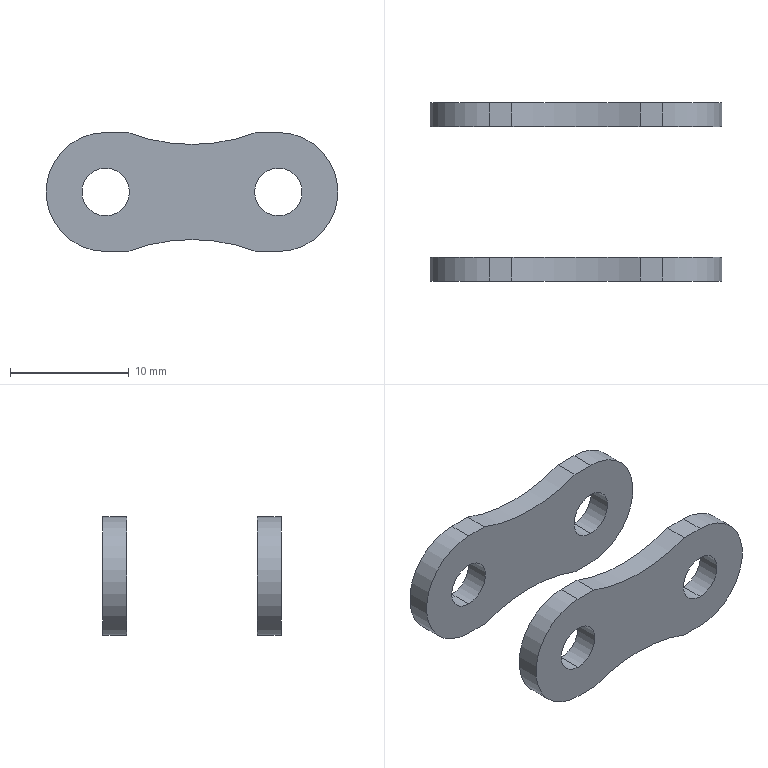Part | SolidWorks | features ICE 2, Extrusion 1 | 2 solids | 30 faces | box 24.52 x 15 x 10 mm | volume 736.592 mm3 | cylinder 18 | plane 12 | commonest cylinder face diameters 4 x8 30 x6 10 x4
STEP:
#1=CARTESIAN_POINT('',(7.26,13.,-4.));
#2=VERTEX_POINT('',#1);
#3=CARTESIAN_POINT('',(12.645,13.,-5.));
#4=VERTEX_POINT('',#3);
#5=CARTESIAN_POINT('',(7.26,13.,-19.));
#6=DIRECTION('',(0.,1.,0.));
#7=DIRECTION('',(0.,0.,1.));
#8=AXIS2_PLACEMENT_3D('',#5,#6,#7);
#9=CIRCLE('',#8,15.);
#10=EDGE_CURVE('',#2,#4,#9,.T.);
#11=ORIENTED_EDGE('',*,*,#10,.F.);
#12=CARTESIAN_POINT('',(7.26,15.,-4.));
#13=VERTEX_POINT('',#12);
#14=CARTESIAN_POINT('',(7.26,0.,-4.));
#15=DIRECTION('',(0.,1.,0.));
#16=VECTOR('',#15,1000.);
#17=LINE('',#14,#16);
#18=EDGE_CURVE('',#2,#13,#17,.T.);
#19=ORIENTED_EDGE('',*,*,#18,.T.);
#20=CARTESIAN_POINT('',(12.645,15.,-5.));
#21=VERTEX_POINT('',#20);
#22=CARTESIAN_POINT('',(7.26,15.,-19.));
#23=DIRECTION('',(0.,1.,0.));
#24=DIRECTION('',(0.,0.,1.));
#25=AXIS2_PLACEMENT_3D('',#22,#23,#24);
#26=CIRCLE('',#25,15.);
#27=EDGE_CURVE('',#13,#21,#26,.T.);
#28=ORIENTED_EDGE('',*,*,#27,.T.);
#29=CARTESIAN_POINT('',(12.645,0.,-5.));
#30=DIRECTION('',(0.,1.,0.));
#31=VECTOR('',#30,1000.);
#32=LINE('',#29,#31);
#33=EDGE_CURVE('',#4,#21,#32,.T.);
#34=ORIENTED_EDGE('',*,*,#33,.F.);
#35=EDGE_LOOP('',(#11,#19,#28,#34));
#36=FACE_OUTER_BOUND('',#35,.T.);
#37=CARTESIAN_POINT('',(7.26,0.,-19.));
#38=DIRECTION('',(0.,1.,0.));
#39=DIRECTION('',(0.,0.,1.));
#40=AXIS2_PLACEMENT_3D('',#37,#38,#39);
#41=CYLINDRICAL_SURFACE('',#40,15.);
#42=ADVANCED_FACE('',(#36),#41,.F.);
#43=CARTESIAN_POINT('',(14.52,15.,-2.));
#44=VERTEX_POINT('',#43);
#45=CARTESIAN_POINT('',(14.52,15.,2.));
#46=VERTEX_POINT('',#45);
#47=CARTESIAN_POINT('',(14.52,15.,0.));
#48=DIRECTION('',(0.,1.,0.));
#49=DIRECTION('',(0.,0.,1.));
#50=AXIS2_PLACEMENT_3D('',#47,#48,#49);
#51=CIRCLE('',#50,2.);
#52=EDGE_CURVE('',#44,#46,#51,.T.);
#53=ORIENTED_EDGE('',*,*,#52,.T.);
#54=CARTESIAN_POINT('',(14.52,13.,2.));
#55=VERTEX_POINT('',#54);
#56=CARTESIAN_POINT('',(14.52,15.,2.));
#57=DIRECTION('',(0.,-1.,0.));
#58=VECTOR('',#57,1000.);
#59=LINE('',#56,#58);
#60=EDGE_CURVE('',#46,#55,#59,.T.);
#61=ORIENTED_EDGE('',*,*,#60,.T.);
#62=CARTESIAN_POINT('',(14.52,13.,-2.));
#63=VERTEX_POINT('',#62);
#64=CARTESIAN_POINT('',(14.52,13.,0.));
#65=DIRECTION('',(0.,1.,0.));
#66=DIRECTION('',(0.,0.,1.));
#67=AXIS2_PLACEMENT_3D('',#64,#65,#66);
#68=CIRCLE('',#67,2.);
#69=EDGE_CURVE('',#63,#55,#68,.T.);
#70=ORIENTED_EDGE('',*,*,#69,.F.);
#71=CARTESIAN_POINT('',(14.52,15.,-2.));
#72=DIRECTION('',(0.,-1.,0.));
#73=VECTOR('',#72,1000.);
#74=LINE('',#71,#73);
#75=EDGE_CURVE('',#44,#63,#74,.T.);
#76=ORIENTED_EDGE('',*,*,#75,.F.);
#77=EDGE_LOOP('',(#53,#61,#70,#76));
#78=FACE_OUTER_BOUND('',#77,.T.);
#79=CARTESIAN_POINT('',(14.52,15.,0.));
#80=DIRECTION('',(0.,-1.,0.));
#81=DIRECTION('',(0.,0.,-1.));
#82=AXIS2_PLACEMENT_3D('',#79,#80,#81);
#83=CYLINDRICAL_SURFACE('',#82,2.);
#84=ADVANCED_FACE('',(#78),#83,.F.);
#85=CARTESIAN_POINT('',(0.,15.,-2.));
#86=VERTEX_POINT('',#85);
#87=CARTESIAN_POINT('',(0.,15.,2.));
#88=VERTEX_POINT('',#87);
#89=CARTESIAN_POINT('',(0.,15.,0.));
#90=DIRECTION('',(0.,1.,0.));
#91=DIRECTION('',(0.,0.,1.));
#92=AXIS2_PLACEMENT_3D('',#89,#90,#91);
#93=CIRCLE('',#92,2.);
#94=EDGE_CURVE('',#86,#88,#93,.T.);
#95=ORIENTED_EDGE('',*,*,#94,.T.);
#96=CARTESIAN_POINT('',(0.,13.,2.));
#97=VERTEX_POINT('',#96);
#98=CARTESIAN_POINT('',(0.,15.,2.));
#99=DIRECTION('',(0.,-1.,0.));
#100=VECTOR('',#99,1000.);
#101=LINE('',#98,#100);
#102=EDGE_CURVE('',#88,#97,#101,.T.);
#103=ORIENTED_EDGE('',*,*,#102,.T.);
#104=CARTESIAN_POINT('',(0.,13.,-2.));
#105=VERTEX_POINT('',#104);
#106=CARTESIAN_POINT('',(0.,13.,0.));
#107=DIRECTION('',(0.,1.,0.));
#108=DIRECTION('',(0.,0.,1.));
#109=AXIS2_PLACEMENT_3D('',#106,#107,#108);
#110=CIRCLE('',#109,2.);
#111=EDGE_CURVE('',#105,#97,#110,.T.);
#112=ORIENTED_EDGE('',*,*,#111,.F.);
#113=CARTESIAN_POINT('',(0.,15.,-2.));
#114=DIRECTION('',(0.,-1.,0.));
#115=VECTOR('',#114,1000.);
#116=LINE('',#113,#115);
#117=EDGE_CURVE('',#86,#105,#116,.T.);
#118=ORIENTED_EDGE('',*,*,#117,.F.);
#119=EDGE_LOOP('',(#95,#103,#112,#118));
#120=FACE_OUTER_BOUND('',#119,.T.);
#121=CARTESIAN_POINT('',(0.,15.,0.));
#122=DIRECTION('',(0.,-1.,0.));
#123=DIRECTION('',(0.,0.,-1.));
#124=AXIS2_PLACEMENT_3D('',#121,#122,#123);
#125=CYLINDRICAL_SURFACE('',#124,2.);
#126=ADVANCED_FACE('',(#120),#125,.F.);
#127=CARTESIAN_POINT('',(0.,13.,5.));
#128=VERTEX_POINT('',#127);
#129=CARTESIAN_POINT('',(1.875,13.,5.));
#130=VERTEX_POINT('',#129);
#131=CARTESIAN_POINT('',(0.,13.,5.));
#132=DIRECTION('',(1.,0.,0.));
#133=VECTOR('',#132,1000.);
#134=LINE('',#131,#133);
#135=EDGE_CURVE('',#128,#130,#134,.T.);
#136=ORIENTED_EDGE('',*,*,#135,.T.);
#137=CARTESIAN_POINT('',(1.875,15.,5.));
#138=VERTEX_POINT('',#137);
#139=CARTESIAN_POINT('',(1.875,0.,5.));
#140=DIRECTION('',(0.,1.,0.));
#141=VECTOR('',#140,1000.);
#142=LINE('',#139,#141);
#143=EDGE_CURVE('',#130,#138,#142,.T.);
#144=ORIENTED_EDGE('',*,*,#143,.T.);
#145=CARTESIAN_POINT('',(0.,15.,5.));
#146=VERTEX_POINT('',#145);
#147=CARTESIAN_POINT('',(0.,15.,5.));
#148=DIRECTION('',(1.,0.,0.));
#149=VECTOR('',#148,1000.);
#150=LINE('',#147,#149);
#151=EDGE_CURVE('',#146,#138,#150,.T.);
#152=ORIENTED_EDGE('',*,*,#151,.F.);
#153=CARTESIAN_POINT('',(0.,15.,5.));
#154=DIRECTION('',(0.,-1.,0.));
#155=VECTOR('',#154,1000.);
#156=LINE('',#153,#155);
#157=EDGE_CURVE('',#146,#128,#156,.T.);
#158=ORIENTED_EDGE('',*,*,#157,.T.);
#159=EDGE_LOOP('',(#136,#144,#152,#158));
#160=FACE_OUTER_BOUND('',#159,.T.);
#161=CARTESIAN_POINT('',(0.,15.,5.));
#162=DIRECTION('',(0.,0.,-1.));
#163=DIRECTION('',(-1.,0.,0.));
#164=AXIS2_PLACEMENT_3D('',#161,#162,#163);
#165=PLANE('',#164);
#166=ADVANCED_FACE('',(#160),#165,.F.);
#167=CARTESIAN_POINT('',(14.52,13.,-5.));
#168=VERTEX_POINT('',#167);
#169=CARTESIAN_POINT('',(0.,13.,-5.));
#170=DIRECTION('',(-1.,0.,0.));
#171=VECTOR('',#170,1000.);
#172=LINE('',#169,#171);
#173=EDGE_CURVE('',#168,#4,#172,.T.);
#174=ORIENTED_EDGE('',*,*,#173,.T.);
#175=ORIENTED_EDGE('',*,*,#33,.T.);
#176=CARTESIAN_POINT('',(14.52,15.,-5.));
#177=VERTEX_POINT('',#176);
#178=CARTESIAN_POINT('',(0.,15.,-5.));
#179=DIRECTION('',(-1.,0.,0.));
#180=VECTOR('',#179,1000.);
#181=LINE('',#178,#180);
#182=EDGE_CURVE('',#177,#21,#181,.T.);
#183=ORIENTED_EDGE('',*,*,#182,.F.);
#184=CARTESIAN_POINT('',(14.52,15.,-5.));
#185=DIRECTION('',(0.,-1.,0.));
#186=VECTOR('',#185,1000.);
#187=LINE('',#184,#186);
#188=EDGE_CURVE('',#177,#168,#187,.T.);
#189=ORIENTED_EDGE('',*,*,#188,.T.);
#190=EDGE_LOOP('',(#174,#175,#183,#189));
#191=FACE_OUTER_BOUND('',#190,.T.);
#192=CARTESIAN_POINT('',(0.,15.,-5.));
#193=DIRECTION('',(0.,0.,1.));
#194=DIRECTION('',(1.,0.,0.));
#195=AXIS2_PLACEMENT_3D('',#192,#193,#194);
#196=PLANE('',#195);
#197=ADVANCED_FACE('',(#191),#196,.F.);
#198=CARTESIAN_POINT('',(1.875,15.,-5.));
#199=VERTEX_POINT('',#198);
#200=CARTESIAN_POINT('',(7.26,15.,-19.));
#201=DIRECTION('',(0.,1.,0.));
#202=DIRECTION('',(0.,0.,1.));
#203=AXIS2_PLACEMENT_3D('',#200,#201,#202);
#204=CIRCLE('',#203,15.);
#205=EDGE_CURVE('',#199,#13,#204,.T.);
#206=ORIENTED_EDGE('',*,*,#205,.F.);
#207=CARTESIAN_POINT('',(0.,15.,-5.));
#208=VERTEX_POINT('',#207);
#209=CARTESIAN_POINT('',(0.,15.,-5.));
#210=DIRECTION('',(-1.,0.,0.));
#211=VECTOR('',#210,1000.);
#212=LINE('',#209,#211);
#213=EDGE_CURVE('',#199,#208,#212,.T.);
#214=ORIENTED_EDGE('',*,*,#213,.T.);
#215=CARTESIAN_POINT('',(0.,15.,0.));
#216=DIRECTION('',(0.,1.,0.));
#217=DIRECTION('',(0.,0.,1.));
#218=AXIS2_PLACEMENT_3D('',#215,#216,#217);
#219=CIRCLE('',#218,5.);
#220=EDGE_CURVE('',#208,#146,#219,.T.);
#221=ORIENTED_EDGE('',*,*,#220,.T.);
#222=ORIENTED_EDGE('',*,*,#151,.T.);
#223=CARTESIAN_POINT('',(12.645,15.,5.));
#224=VERTEX_POINT('',#223);
#225=CARTESIAN_POINT('',(7.26,15.,19.));
#226=DIRECTION('',(0.,1.,0.));
#227=DIRECTION('',(0.,0.,1.));
#228=AXIS2_PLACEMENT_3D('',#225,#226,#227);
#229=CIRCLE('',#228,15.);
#230=EDGE_CURVE('',#224,#138,#229,.T.);
#231=ORIENTED_EDGE('',*,*,#230,.F.);
#232=CARTESIAN_POINT('',(14.52,15.,5.));
#233=VERTEX_POINT('',#232);
#234=CARTESIAN_POINT('',(0.,15.,5.));
#235=DIRECTION('',(1.,0.,0.));
#236=VECTOR('',#235,1000.);
#237=LINE('',#234,#236);
#238=EDGE_CURVE('',#224,#233,#237,.T.);
#239=ORIENTED_EDGE('',*,*,#238,.T.);
#240=CARTESIAN_POINT('',(14.52,15.,0.));
#241=DIRECTION('',(0.,1.,0.));
#242=DIRECTION('',(0.,0.,1.));
#243=AXIS2_PLACEMENT_3D('',#240,#241,#242);
#244=CIRCLE('',#243,5.);
#245=EDGE_CURVE('',#233,#177,#244,.T.);
#246=ORIENTED_EDGE('',*,*,#245,.T.);
#247=ORIENTED_EDGE('',*,*,#182,.T.);
#248=ORIENTED_EDGE('',*,*,#27,.F.);
#249=EDGE_LOOP('',(#206,#214,#221,#222,#231,#239,#246,#247,#248));
#250=FACE_OUTER_BOUND('',#249,.T.);
#251=ORIENTED_EDGE('',*,*,#94,.F.);
#252=CARTESIAN_POINT('',(0.,15.,0.));
#253=DIRECTION('',(0.,1.,0.));
#254=DIRECTION('',(0.,0.,1.));
#255=AXIS2_PLACEMENT_3D('',#252,#253,#254);
#256=CIRCLE('',#255,2.);
#257=EDGE_CURVE('',#88,#86,#256,.T.);
#258=ORIENTED_EDGE('',*,*,#257,.F.);
#259=EDGE_LOOP('',(#251,#258));
#260=FACE_BOUND('',#259,.T.);
#261=ORIENTED_EDGE('',*,*,#52,.F.);
#262=CARTESIAN_POINT('',(14.52,15.,0.));
#263=DIRECTION('',(0.,1.,0.));
#264=DIRECTION('',(0.,0.,1.));
#265=AXIS2_PLACEMENT_3D('',#262,#263,#264);
#266=CIRCLE('',#265,2.);
#267=EDGE_CURVE('',#46,#44,#266,.T.);
#268=ORIENTED_EDGE('',*,*,#267,.F.);
#269=EDGE_LOOP('',(#261,#268));
#270=FACE_BOUND('',#269,.T.);
#271=CARTESIAN_POINT('',(0.,15.,0.));
#272=DIRECTION('',(0.,1.,0.));
#273=DIRECTION('',(0.,0.,1.));
#274=AXIS2_PLACEMENT_3D('',#271,#272,#273);
#275=PLANE('',#274);
#276=ADVANCED_FACE('',(#250,#260,#270),#275,.T.);
#277=CARTESIAN_POINT('',(0.,13.,-5.));
#278=VERTEX_POINT('',#277);
#279=CARTESIAN_POINT('',(0.,15.,-5.));
#280=DIRECTION('',(0.,-1.,0.));
#281=VECTOR('',#280,1000.);
#282=LINE('',#279,#281);
#283=EDGE_CURVE('',#208,#278,#282,.T.);
#284=ORIENTED_EDGE('',*,*,#283,.T.);
#285=CARTESIAN_POINT('',(0.,13.,0.));
#286=DIRECTION('',(0.,1.,0.));
#287=DIRECTION('',(0.,0.,1.));
#288=AXIS2_PLACEMENT_3D('',#285,#286,#287);
#289=CIRCLE('',#288,5.);
#290=EDGE_CURVE('',#278,#128,#289,.T.);
#291=ORIENTED_EDGE('',*,*,#290,.T.);
#292=ORIENTED_EDGE('',*,*,#157,.F.);
#293=ORIENTED_EDGE('',*,*,#220,.F.);
#294=EDGE_LOOP('',(#284,#291,#292,#293));
#295=FACE_OUTER_BOUND('',#294,.T.);
#296=CARTESIAN_POINT('',(0.,15.,0.));
#297=DIRECTION('',(0.,-1.,0.));
#298=DIRECTION('',(0.,0.,-1.));
#299=AXIS2_PLACEMENT_3D('',#296,#297,#298);
#300=CYLINDRICAL_SURFACE('',#299,5.);
#301=ADVANCED_FACE('',(#295),#300,.T.);
#302=ORIENTED_EDGE('',*,*,#238,.F.);
#303=CARTESIAN_POINT('',(12.645,13.,5.));
#304=VERTEX_POINT('',#303);
#305=CARTESIAN_POINT('',(12.645,0.,5.));
#306=DIRECTION('',(0.,-1.,0.));
#307=VECTOR('',#306,1000.);
#308=LINE('',#305,#307);
#309=EDGE_CURVE('',#224,#304,#308,.T.);
#310=ORIENTED_EDGE('',*,*,#309,.T.);
#311=CARTESIAN_POINT('',(14.52,13.,5.));
#312=VERTEX_POINT('',#311);
#313=CARTESIAN_POINT('',(0.,13.,5.));
#314=DIRECTION('',(1.,0.,0.));
#315=VECTOR('',#314,1000.);
#316=LINE('',#313,#315);
#317=EDGE_CURVE('',#304,#312,#316,.T.);
#318=ORIENTED_EDGE('',*,*,#317,.T.);
#319=CARTESIAN_POINT('',(14.52,15.,5.));
#320=DIRECTION('',(0.,-1.,0.));
#321=VECTOR('',#320,1000.);
#322=LINE('',#319,#321);
#323=EDGE_CURVE('',#233,#312,#322,.T.);
#324=ORIENTED_EDGE('',*,*,#323,.F.);
#325=EDGE_LOOP('',(#302,#310,#318,#324));
#326=FACE_OUTER_BOUND('',#325,.T.);
#327=CARTESIAN_POINT('',(0.,15.,5.));
#328=DIRECTION('',(0.,0.,-1.));
#329=DIRECTION('',(-1.,0.,0.));
#330=AXIS2_PLACEMENT_3D('',#327,#328,#329);
#331=PLANE('',#330);
#332=ADVANCED_FACE('',(#326),#331,.F.);
#333=ORIENTED_EDGE('',*,*,#323,.T.);
#334=CARTESIAN_POINT('',(14.52,13.,0.));
#335=DIRECTION('',(0.,1.,0.));
#336=DIRECTION('',(0.,0.,1.));
#337=AXIS2_PLACEMENT_3D('',#334,#335,#336);
#338=CIRCLE('',#337,5.);
#339=EDGE_CURVE('',#312,#168,#338,.T.);
#340=ORIENTED_EDGE('',*,*,#339,.T.);
#341=ORIENTED_EDGE('',*,*,#188,.F.);
#342=ORIENTED_EDGE('',*,*,#245,.F.);
#343=EDGE_LOOP('',(#333,#340,#341,#342));
#344=FACE_OUTER_BOUND('',#343,.T.);
#345=CARTESIAN_POINT('',(14.52,15.,0.));
#346=DIRECTION('',(0.,-1.,0.));
#347=DIRECTION('',(0.,0.,-1.));
#348=AXIS2_PLACEMENT_3D('',#345,#346,#347);
#349=CYLINDRICAL_SURFACE('',#348,5.);
#350=ADVANCED_FACE('',(#344),#349,.T.);
#351=ORIENTED_EDGE('',*,*,#213,.F.);
#352=CARTESIAN_POINT('',(1.875,13.,-5.));
#353=VERTEX_POINT('',#352);
#354=CARTESIAN_POINT('',(1.875,0.,-5.));
#355=DIRECTION('',(0.,-1.,0.));
#356=VECTOR('',#355,1000.);
#357=LINE('',#354,#356);
#358=EDGE_CURVE('',#199,#353,#357,.T.);
#359=ORIENTED_EDGE('',*,*,#358,.T.);
#360=CARTESIAN_POINT('',(0.,13.,-5.));
#361=DIRECTION('',(-1.,0.,0.));
#362=VECTOR('',#361,1000.);
#363=LINE('',#360,#362);
#364=EDGE_CURVE('',#353,#278,#363,.T.);
#365=ORIENTED_EDGE('',*,*,#364,.T.);
#366=ORIENTED_EDGE('',*,*,#283,.F.);
#367=EDGE_LOOP('',(#351,#359,#365,#366));
#368=FACE_OUTER_BOUND('',#367,.T.);
#369=CARTESIAN_POINT('',(0.,15.,-5.));
#370=DIRECTION('',(0.,0.,1.));
#371=DIRECTION('',(1.,0.,0.));
#372=AXIS2_PLACEMENT_3D('',#369,#370,#371);
#373=PLANE('',#372);
#374=ADVANCED_FACE('',(#368),#373,.F.);
#375=ORIENTED_EDGE('',*,*,#102,.F.);
#376=ORIENTED_EDGE('',*,*,#257,.T.);
#377=ORIENTED_EDGE('',*,*,#117,.T.);
#378=CARTESIAN_POINT('',(0.,13.,0.));
#379=DIRECTION('',(0.,1.,0.));
#380=DIRECTION('',(0.,0.,1.));
#381=AXIS2_PLACEMENT_3D('',#378,#379,#380);
#382=CIRCLE('',#381,2.);
#383=EDGE_CURVE('',#97,#105,#382,.T.);
#384=ORIENTED_EDGE('',*,*,#383,.F.);
#385=EDGE_LOOP('',(#375,#376,#377,#384));
#386=FACE_OUTER_BOUND('',#385,.T.);
#387=CARTESIAN_POINT('',(0.,15.,0.));
#388=DIRECTION('',(0.,-1.,0.));
#389=DIRECTION('',(0.,0.,-1.));
#390=AXIS2_PLACEMENT_3D('',#387,#388,#389);
#391=CYLINDRICAL_SURFACE('',#390,2.);
#392=ADVANCED_FACE('',(#386),#391,.F.);
#393=ORIENTED_EDGE('',*,*,#60,.F.);
#394=ORIENTED_EDGE('',*,*,#267,.T.);
#395=ORIENTED_EDGE('',*,*,#75,.T.);
#396=CARTESIAN_POINT('',(14.52,13.,0.));
#397=DIRECTION('',(0.,1.,0.));
#398=DIRECTION('',(0.,0.,1.));
#399=AXIS2_PLACEMENT_3D('',#396,#397,#398);
#400=CIRCLE('',#399,2.);
#401=EDGE_CURVE('',#55,#63,#400,.T.);
#402=ORIENTED_EDGE('',*,*,#401,.F.);
#403=EDGE_LOOP('',(#393,#394,#395,#402));
#404=FACE_OUTER_BOUND('',#403,.T.);
#405=CARTESIAN_POINT('',(14.52,15.,0.));
#406=DIRECTION('',(0.,-1.,0.));
#407=DIRECTION('',(0.,0.,-1.));
#408=AXIS2_PLACEMENT_3D('',#405,#406,#407);
#409=CYLINDRICAL_SURFACE('',#408,2.);
#410=ADVANCED_FACE('',(#404),#409,.F.);
#411=ORIENTED_EDGE('',*,*,#69,.T.);
#412=ORIENTED_EDGE('',*,*,#401,.T.);
#413=EDGE_LOOP('',(#411,#412));
#414=FACE_BOUND('',#413,.T.);
#415=ORIENTED_EDGE('',*,*,#111,.T.);
#416=ORIENTED_EDGE('',*,*,#383,.T.);
#417=EDGE_LOOP('',(#415,#416));
#418=FACE_BOUND('',#417,.T.);
#419=ORIENTED_EDGE('',*,*,#364,.F.);
#420=CARTESIAN_POINT('',(7.26,13.,-19.));
#421=DIRECTION('',(0.,1.,0.));
#422=DIRECTION('',(0.,0.,1.));
#423=AXIS2_PLACEMENT_3D('',#420,#421,#422);
#424=CIRCLE('',#423,15.);
#425=EDGE_CURVE('',#353,#2,#424,.T.);
#426=ORIENTED_EDGE('',*,*,#425,.T.);
#427=ORIENTED_EDGE('',*,*,#10,.T.);
#428=ORIENTED_EDGE('',*,*,#173,.F.);
#429=ORIENTED_EDGE('',*,*,#339,.F.);
#430=ORIENTED_EDGE('',*,*,#317,.F.);
#431=CARTESIAN_POINT('',(7.26,13.,19.));
#432=DIRECTION('',(0.,1.,0.));
#433=DIRECTION('',(0.,0.,1.));
#434=AXIS2_PLACEMENT_3D('',#431,#432,#433);
#435=CIRCLE('',#434,15.);
#436=EDGE_CURVE('',#304,#130,#435,.T.);
#437=ORIENTED_EDGE('',*,*,#436,.T.);
#438=ORIENTED_EDGE('',*,*,#135,.F.);
#439=ORIENTED_EDGE('',*,*,#290,.F.);
#440=EDGE_LOOP('',(#419,#426,#427,#428,#429,#430,#437,#438,#439));
#441=FACE_OUTER_BOUND('',#440,.T.);
#442=CARTESIAN_POINT('',(0.,13.,0.));
#443=DIRECTION('',(0.,1.,0.));
#444=DIRECTION('',(0.,0.,1.));
#445=AXIS2_PLACEMENT_3D('',#442,#443,#444);
#446=PLANE('',#445);
#447=ADVANCED_FACE('',(#414,#418,#441),#446,.F.);
#448=ORIENTED_EDGE('',*,*,#436,.F.);
#449=ORIENTED_EDGE('',*,*,#309,.F.);
#450=ORIENTED_EDGE('',*,*,#230,.T.);
#451=ORIENTED_EDGE('',*,*,#143,.F.);
#452=EDGE_LOOP('',(#448,#449,#450,#451));
#453=FACE_OUTER_BOUND('',#452,.T.);
#454=CARTESIAN_POINT('',(7.26,0.,19.));
#455=DIRECTION('',(0.,1.,0.));
#456=DIRECTION('',(0.,0.,1.));
#457=AXIS2_PLACEMENT_3D('',#454,#455,#456);
#458=CYLINDRICAL_SURFACE('',#457,15.);
#459=ADVANCED_FACE('',(#453),#458,.F.);
#460=ORIENTED_EDGE('',*,*,#18,.F.);
#461=ORIENTED_EDGE('',*,*,#425,.F.);
#462=ORIENTED_EDGE('',*,*,#358,.F.);
#463=ORIENTED_EDGE('',*,*,#205,.T.);
#464=EDGE_LOOP('',(#460,#461,#462,#463));
#465=FACE_OUTER_BOUND('',#464,.T.);
#466=CARTESIAN_POINT('',(7.26,0.,-19.));
#467=DIRECTION('',(0.,1.,0.));
#468=DIRECTION('',(0.,0.,1.));
#469=AXIS2_PLACEMENT_3D('',#466,#467,#468);
#470=CYLINDRICAL_SURFACE('',#469,15.);
#471=ADVANCED_FACE('',(#465),#470,.F.);
#472=CLOSED_SHELL('',(#42,#84,#126,#166,#197,#276,#301,#332,#350,#374,#392,#410,#447,#459,#471));
#473=MANIFOLD_SOLID_BREP('',#472);
#474=CARTESIAN_POINT('',(7.26,0.,-4.));
#475=VERTEX_POINT('',#474);
#476=CARTESIAN_POINT('',(12.645,0.,-5.));
#477=VERTEX_POINT('',#476);
#478=CARTESIAN_POINT('',(7.26,0.,-19.));
#479=DIRECTION('',(0.,1.,0.));
#480=DIRECTION('',(0.,0.,1.));
#481=AXIS2_PLACEMENT_3D('',#478,#479,#480);
#482=CIRCLE('',#481,15.);
#483=EDGE_CURVE('',#475,#477,#482,.T.);
#484=ORIENTED_EDGE('',*,*,#483,.F.);
#485=CARTESIAN_POINT('',(7.26,2.,-4.));
#486=VERTEX_POINT('',#485);
#487=CARTESIAN_POINT('',(7.26,0.,-4.));
#488=DIRECTION('',(0.,1.,0.));
#489=VECTOR('',#488,1000.);
#490=LINE('',#487,#489);
#491=EDGE_CURVE('',#475,#486,#490,.T.);
#492=ORIENTED_EDGE('',*,*,#491,.T.);
#493=CARTESIAN_POINT('',(12.645,2.,-5.));
#494=VERTEX_POINT('',#493);
#495=CARTESIAN_POINT('',(7.26,2.,-19.));
#496=DIRECTION('',(0.,1.,0.));
#497=DIRECTION('',(0.,0.,1.));
#498=AXIS2_PLACEMENT_3D('',#495,#496,#497);
#499=CIRCLE('',#498,15.);
#500=EDGE_CURVE('',#486,#494,#499,.T.);
#501=ORIENTED_EDGE('',*,*,#500,.T.);
#502=CARTESIAN_POINT('',(12.645,0.,-5.));
#503=DIRECTION('',(0.,1.,0.));
#504=VECTOR('',#503,1000.);
#505=LINE('',#502,#504);
#506=EDGE_CURVE('',#477,#494,#505,.T.);
#507=ORIENTED_EDGE('',*,*,#506,.F.);
#508=EDGE_LOOP('',(#484,#492,#501,#507));
#509=FACE_OUTER_BOUND('',#508,.T.);
#510=CARTESIAN_POINT('',(7.26,0.,-19.));
#511=DIRECTION('',(0.,1.,0.));
#512=DIRECTION('',(0.,0.,1.));
#513=AXIS2_PLACEMENT_3D('',#510,#511,#512);
#514=CYLINDRICAL_SURFACE('',#513,15.);
#515=ADVANCED_FACE('',(#509),#514,.F.);
#516=CARTESIAN_POINT('',(14.52,2.,-2.));
#517=VERTEX_POINT('',#516);
#518=CARTESIAN_POINT('',(14.52,2.,2.));
#519=VERTEX_POINT('',#518);
#520=CARTESIAN_POINT('',(14.52,2.,0.));
#521=DIRECTION('',(0.,1.,0.));
#522=DIRECTION('',(0.,0.,1.));
#523=AXIS2_PLACEMENT_3D('',#520,#521,#522);
#524=CIRCLE('',#523,2.);
#525=EDGE_CURVE('',#517,#519,#524,.T.);
#526=ORIENTED_EDGE('',*,*,#525,.T.);
#527=CARTESIAN_POINT('',(14.52,0.,2.));
#528=VERTEX_POINT('',#527);
#529=CARTESIAN_POINT('',(14.52,15.,2.));
#530=DIRECTION('',(0.,-1.,0.));
#531=VECTOR('',#530,1000.);
#532=LINE('',#529,#531);
#533=EDGE_CURVE('',#519,#528,#532,.T.);
#534=ORIENTED_EDGE('',*,*,#533,.T.);
#535=CARTESIAN_POINT('',(14.52,0.,-2.));
#536=VERTEX_POINT('',#535);
#537=CARTESIAN_POINT('',(14.52,0.,0.));
#538=DIRECTION('',(0.,1.,0.));
#539=DIRECTION('',(0.,0.,1.));
#540=AXIS2_PLACEMENT_3D('',#537,#538,#539);
#541=CIRCLE('',#540,2.);
#542=EDGE_CURVE('',#536,#528,#541,.T.);
#543=ORIENTED_EDGE('',*,*,#542,.F.);
#544=CARTESIAN_POINT('',(14.52,15.,-2.));
#545=DIRECTION('',(0.,-1.,0.));
#546=VECTOR('',#545,1000.);
#547=LINE('',#544,#546);
#548=EDGE_CURVE('',#517,#536,#547,.T.);
#549=ORIENTED_EDGE('',*,*,#548,.F.);
#550=EDGE_LOOP('',(#526,#534,#543,#549));
#551=FACE_OUTER_BOUND('',#550,.T.);
#552=CARTESIAN_POINT('',(14.52,15.,0.));
#553=DIRECTION('',(0.,-1.,0.));
#554=DIRECTION('',(0.,0.,-1.));
#555=AXIS2_PLACEMENT_3D('',#552,#553,#554);
#556=CYLINDRICAL_SURFACE('',#555,2.);
#557=ADVANCED_FACE('',(#551),#556,.F.);
#558=CARTESIAN_POINT('',(0.,2.,-2.));
#559=VERTEX_POINT('',#558);
#560=CARTESIAN_POINT('',(0.,2.,2.));
#561=VERTEX_POINT('',#560);
#562=CARTESIAN_POINT('',(0.,2.,0.));
#563=DIRECTION('',(0.,1.,0.));
#564=DIRECTION('',(0.,0.,1.));
#565=AXIS2_PLACEMENT_3D('',#562,#563,#564);
#566=CIRCLE('',#565,2.);
#567=EDGE_CURVE('',#559,#561,#566,.T.);
#568=ORIENTED_EDGE('',*,*,#567,.T.);
#569=CARTESIAN_POINT('',(0.,0.,2.));
#570=VERTEX_POINT('',#569);
#571=CARTESIAN_POINT('',(0.,15.,2.));
#572=DIRECTION('',(0.,-1.,0.));
#573=VECTOR('',#572,1000.);
#574=LINE('',#571,#573);
#575=EDGE_CURVE('',#561,#570,#574,.T.);
#576=ORIENTED_EDGE('',*,*,#575,.T.);
#577=CARTESIAN_POINT('',(0.,0.,-2.));
#578=VERTEX_POINT('',#577);
#579=CARTESIAN_POINT('',(0.,0.,0.));
#580=DIRECTION('',(0.,1.,0.));
#581=DIRECTION('',(0.,0.,1.));
#582=AXIS2_PLACEMENT_3D('',#579,#580,#581);
#583=CIRCLE('',#582,2.);
#584=EDGE_CURVE('',#578,#570,#583,.T.);
#585=ORIENTED_EDGE('',*,*,#584,.F.);
#586=CARTESIAN_POINT('',(0.,15.,-2.));
#587=DIRECTION('',(0.,-1.,0.));
#588=VECTOR('',#587,1000.);
#589=LINE('',#586,#588);
#590=EDGE_CURVE('',#559,#578,#589,.T.);
#591=ORIENTED_EDGE('',*,*,#590,.F.);
#592=EDGE_LOOP('',(#568,#576,#585,#591));
#593=FACE_OUTER_BOUND('',#592,.T.);
#594=CARTESIAN_POINT('',(0.,15.,0.));
#595=DIRECTION('',(0.,-1.,0.));
#596=DIRECTION('',(0.,0.,-1.));
#597=AXIS2_PLACEMENT_3D('',#594,#595,#596);
#598=CYLINDRICAL_SURFACE('',#597,2.);
#599=ADVANCED_FACE('',(#593),#598,.F.);
#600=CARTESIAN_POINT('',(14.52,0.,-5.));
#601=VERTEX_POINT('',#600);
#602=CARTESIAN_POINT('',(0.,0.,-5.));
#603=DIRECTION('',(-1.,0.,0.));
#604=VECTOR('',#603,1000.);
#605=LINE('',#602,#604);
#606=EDGE_CURVE('',#601,#477,#605,.T.);
#607=ORIENTED_EDGE('',*,*,#606,.T.);
#608=ORIENTED_EDGE('',*,*,#506,.T.);
#609=CARTESIAN_POINT('',(14.52,2.,-5.));
#610=VERTEX_POINT('',#609);
#611=CARTESIAN_POINT('',(0.,2.,-5.));
#612=DIRECTION('',(-1.,0.,0.));
#613=VECTOR('',#612,1000.);
#614=LINE('',#611,#613);
#615=EDGE_CURVE('',#610,#494,#614,.T.);
#616=ORIENTED_EDGE('',*,*,#615,.F.);
#617=CARTESIAN_POINT('',(14.52,15.,-5.));
#618=DIRECTION('',(0.,-1.,0.));
#619=VECTOR('',#618,1000.);
#620=LINE('',#617,#619);
#621=EDGE_CURVE('',#610,#601,#620,.T.);
#622=ORIENTED_EDGE('',*,*,#621,.T.);
#623=EDGE_LOOP('',(#607,#608,#616,#622));
#624=FACE_OUTER_BOUND('',#623,.T.);
#625=CARTESIAN_POINT('',(0.,15.,-5.));
#626=DIRECTION('',(0.,0.,1.));
#627=DIRECTION('',(1.,0.,0.));
#628=AXIS2_PLACEMENT_3D('',#625,#626,#627);
#629=PLANE('',#628);
#630=ADVANCED_FACE('',(#624),#629,.F.);
#631=CARTESIAN_POINT('',(0.,0.,5.));
#632=VERTEX_POINT('',#631);
#633=CARTESIAN_POINT('',(1.875,0.,5.));
#634=VERTEX_POINT('',#633);
#635=CARTESIAN_POINT('',(0.,0.,5.));
#636=DIRECTION('',(1.,0.,0.));
#637=VECTOR('',#636,1000.);
#638=LINE('',#635,#637);
#639=EDGE_CURVE('',#632,#634,#638,.T.);
#640=ORIENTED_EDGE('',*,*,#639,.T.);
#641=CARTESIAN_POINT('',(1.875,2.,5.));
#642=VERTEX_POINT('',#641);
#643=CARTESIAN_POINT('',(1.875,0.,5.));
#644=DIRECTION('',(0.,1.,0.));
#645=VECTOR('',#644,1000.);
#646=LINE('',#643,#645);
#647=EDGE_CURVE('',#634,#642,#646,.T.);
#648=ORIENTED_EDGE('',*,*,#647,.T.);
#649=CARTESIAN_POINT('',(0.,2.,5.));
#650=VERTEX_POINT('',#649);
#651=CARTESIAN_POINT('',(0.,2.,5.));
#652=DIRECTION('',(1.,0.,0.));
#653=VECTOR('',#652,1000.);
#654=LINE('',#651,#653);
#655=EDGE_CURVE('',#650,#642,#654,.T.);
#656=ORIENTED_EDGE('',*,*,#655,.F.);
#657=CARTESIAN_POINT('',(0.,15.,5.));
#658=DIRECTION('',(0.,-1.,0.));
#659=VECTOR('',#658,1000.);
#660=LINE('',#657,#659);
#661=EDGE_CURVE('',#650,#632,#660,.T.);
#662=ORIENTED_EDGE('',*,*,#661,.T.);
#663=EDGE_LOOP('',(#640,#648,#656,#662));
#664=FACE_OUTER_BOUND('',#663,.T.);
#665=CARTESIAN_POINT('',(0.,15.,5.));
#666=DIRECTION('',(0.,0.,-1.));
#667=DIRECTION('',(-1.,0.,0.));
#668=AXIS2_PLACEMENT_3D('',#665,#666,#667);
#669=PLANE('',#668);
#670=ADVANCED_FACE('',(#664),#669,.F.);
#671=ORIENTED_EDGE('',*,*,#575,.F.);
#672=CARTESIAN_POINT('',(0.,2.,0.));
#673=DIRECTION('',(0.,1.,0.));
#674=DIRECTION('',(0.,0.,1.));
#675=AXIS2_PLACEMENT_3D('',#672,#673,#674);
#676=CIRCLE('',#675,2.);
#677=EDGE_CURVE('',#561,#559,#676,.T.);
#678=ORIENTED_EDGE('',*,*,#677,.T.);
#679=ORIENTED_EDGE('',*,*,#590,.T.);
#680=CARTESIAN_POINT('',(0.,0.,0.));
#681=DIRECTION('',(0.,1.,0.));
#682=DIRECTION('',(0.,0.,1.));
#683=AXIS2_PLACEMENT_3D('',#680,#681,#682);
#684=CIRCLE('',#683,2.);
#685=EDGE_CURVE('',#570,#578,#684,.T.);
#686=ORIENTED_EDGE('',*,*,#685,.F.);
#687=EDGE_LOOP('',(#671,#678,#679,#686));
#688=FACE_OUTER_BOUND('',#687,.T.);
#689=CARTESIAN_POINT('',(0.,15.,0.));
#690=DIRECTION('',(0.,-1.,0.));
#691=DIRECTION('',(0.,0.,-1.));
#692=AXIS2_PLACEMENT_3D('',#689,#690,#691);
#693=CYLINDRICAL_SURFACE('',#692,2.);
#694=ADVANCED_FACE('',(#688),#693,.F.);
#695=CARTESIAN_POINT('',(1.875,2.,-5.));
#696=VERTEX_POINT('',#695);
#697=CARTESIAN_POINT('',(0.,2.,-5.));
#698=VERTEX_POINT('',#697);
#699=CARTESIAN_POINT('',(0.,2.,-5.));
#700=DIRECTION('',(-1.,0.,0.));
#701=VECTOR('',#700,1000.);
#702=LINE('',#699,#701);
#703=EDGE_CURVE('',#696,#698,#702,.T.);
#704=ORIENTED_EDGE('',*,*,#703,.F.);
#705=CARTESIAN_POINT('',(1.875,0.,-5.));
#706=VERTEX_POINT('',#705);
#707=CARTESIAN_POINT('',(1.875,0.,-5.));
#708=DIRECTION('',(0.,-1.,0.));
#709=VECTOR('',#708,1000.);
#710=LINE('',#707,#709);
#711=EDGE_CURVE('',#696,#706,#710,.T.);
#712=ORIENTED_EDGE('',*,*,#711,.T.);
#713=CARTESIAN_POINT('',(0.,0.,-5.));
#714=VERTEX_POINT('',#713);
#715=CARTESIAN_POINT('',(0.,0.,-5.));
#716=DIRECTION('',(-1.,0.,0.));
#717=VECTOR('',#716,1000.);
#718=LINE('',#715,#717);
#719=EDGE_CURVE('',#706,#714,#718,.T.);
#720=ORIENTED_EDGE('',*,*,#719,.T.);
#721=CARTESIAN_POINT('',(0.,15.,-5.));
#722=DIRECTION('',(0.,-1.,0.));
#723=VECTOR('',#722,1000.);
#724=LINE('',#721,#723);
#725=EDGE_CURVE('',#698,#714,#724,.T.);
#726=ORIENTED_EDGE('',*,*,#725,.F.);
#727=EDGE_LOOP('',(#704,#712,#720,#726));
#728=FACE_OUTER_BOUND('',#727,.T.);
#729=CARTESIAN_POINT('',(0.,15.,-5.));
#730=DIRECTION('',(0.,0.,1.));
#731=DIRECTION('',(1.,0.,0.));
#732=AXIS2_PLACEMENT_3D('',#729,#730,#731);
#733=PLANE('',#732);
#734=ADVANCED_FACE('',(#728),#733,.F.);
#735=CARTESIAN_POINT('',(14.52,2.,5.));
#736=VERTEX_POINT('',#735);
#737=CARTESIAN_POINT('',(14.52,2.,0.));
#738=DIRECTION('',(0.,1.,0.));
#739=DIRECTION('',(0.,0.,1.));
#740=AXIS2_PLACEMENT_3D('',#737,#738,#739);
#741=CIRCLE('',#740,5.);
#742=EDGE_CURVE('',#736,#610,#741,.T.);
#743=ORIENTED_EDGE('',*,*,#742,.F.);
#744=CARTESIAN_POINT('',(14.52,0.,5.));
#745=VERTEX_POINT('',#744);
#746=CARTESIAN_POINT('',(14.52,15.,5.));
#747=DIRECTION('',(0.,-1.,0.));
#748=VECTOR('',#747,1000.);
#749=LINE('',#746,#748);
#750=EDGE_CURVE('',#736,#745,#749,.T.);
#751=ORIENTED_EDGE('',*,*,#750,.T.);
#752=CARTESIAN_POINT('',(14.52,0.,0.));
#753=DIRECTION('',(0.,1.,0.));
#754=DIRECTION('',(0.,0.,1.));
#755=AXIS2_PLACEMENT_3D('',#752,#753,#754);
#756=CIRCLE('',#755,5.);
#757=EDGE_CURVE('',#745,#601,#756,.T.);
#758=ORIENTED_EDGE('',*,*,#757,.T.);
#759=ORIENTED_EDGE('',*,*,#621,.F.);
#760=EDGE_LOOP('',(#743,#751,#758,#759));
#761=FACE_OUTER_BOUND('',#760,.T.);
#762=CARTESIAN_POINT('',(14.52,15.,0.));
#763=DIRECTION('',(0.,-1.,0.));
#764=DIRECTION('',(0.,0.,-1.));
#765=AXIS2_PLACEMENT_3D('',#762,#763,#764);
#766=CYLINDRICAL_SURFACE('',#765,5.);
#767=ADVANCED_FACE('',(#761),#766,.T.);
#768=CARTESIAN_POINT('',(12.645,2.,5.));
#769=VERTEX_POINT('',#768);
#770=CARTESIAN_POINT('',(0.,2.,5.));
#771=DIRECTION('',(1.,0.,0.));
#772=VECTOR('',#771,1000.);
#773=LINE('',#770,#772);
#774=EDGE_CURVE('',#769,#736,#773,.T.);
#775=ORIENTED_EDGE('',*,*,#774,.F.);
#776=CARTESIAN_POINT('',(12.645,0.,5.));
#777=VERTEX_POINT('',#776);
#778=CARTESIAN_POINT('',(12.645,0.,5.));
#779=DIRECTION('',(0.,-1.,0.));
#780=VECTOR('',#779,1000.);
#781=LINE('',#778,#780);
#782=EDGE_CURVE('',#769,#777,#781,.T.);
#783=ORIENTED_EDGE('',*,*,#782,.T.);
#784=CARTESIAN_POINT('',(0.,0.,5.));
#785=DIRECTION('',(1.,0.,0.));
#786=VECTOR('',#785,1000.);
#787=LINE('',#784,#786);
#788=EDGE_CURVE('',#777,#745,#787,.T.);
#789=ORIENTED_EDGE('',*,*,#788,.T.);
#790=ORIENTED_EDGE('',*,*,#750,.F.);
#791=EDGE_LOOP('',(#775,#783,#789,#790));
#792=FACE_OUTER_BOUND('',#791,.T.);
#793=CARTESIAN_POINT('',(0.,15.,5.));
#794=DIRECTION('',(0.,0.,-1.));
#795=DIRECTION('',(-1.,0.,0.));
#796=AXIS2_PLACEMENT_3D('',#793,#794,#795);
#797=PLANE('',#796);
#798=ADVANCED_FACE('',(#792),#797,.F.);
#799=CARTESIAN_POINT('',(0.,2.,0.));
#800=DIRECTION('',(0.,1.,0.));
#801=DIRECTION('',(0.,0.,1.));
#802=AXIS2_PLACEMENT_3D('',#799,#800,#801);
#803=CIRCLE('',#802,5.);
#804=EDGE_CURVE('',#698,#650,#803,.T.);
#805=ORIENTED_EDGE('',*,*,#804,.F.);
#806=ORIENTED_EDGE('',*,*,#725,.T.);
#807=CARTESIAN_POINT('',(0.,0.,0.));
#808=DIRECTION('',(0.,1.,0.));
#809=DIRECTION('',(0.,0.,1.));
#810=AXIS2_PLACEMENT_3D('',#807,#808,#809);
#811=CIRCLE('',#810,5.);
#812=EDGE_CURVE('',#714,#632,#811,.T.);
#813=ORIENTED_EDGE('',*,*,#812,.T.);
#814=ORIENTED_EDGE('',*,*,#661,.F.);
#815=EDGE_LOOP('',(#805,#806,#813,#814));
#816=FACE_OUTER_BOUND('',#815,.T.);
#817=CARTESIAN_POINT('',(0.,15.,0.));
#818=DIRECTION('',(0.,-1.,0.));
#819=DIRECTION('',(0.,0.,-1.));
#820=AXIS2_PLACEMENT_3D('',#817,#818,#819);
#821=CYLINDRICAL_SURFACE('',#820,5.);
#822=ADVANCED_FACE('',(#816),#821,.T.);
#823=ORIENTED_EDGE('',*,*,#719,.F.);
#824=CARTESIAN_POINT('',(7.26,0.,-19.));
#825=DIRECTION('',(0.,1.,0.));
#826=DIRECTION('',(0.,0.,1.));
#827=AXIS2_PLACEMENT_3D('',#824,#825,#826);
#828=CIRCLE('',#827,15.);
#829=EDGE_CURVE('',#706,#475,#828,.T.);
#830=ORIENTED_EDGE('',*,*,#829,.T.);
#831=ORIENTED_EDGE('',*,*,#483,.T.);
#832=ORIENTED_EDGE('',*,*,#606,.F.);
#833=ORIENTED_EDGE('',*,*,#757,.F.);
#834=ORIENTED_EDGE('',*,*,#788,.F.);
#835=CARTESIAN_POINT('',(7.26,0.,19.));
#836=DIRECTION('',(0.,1.,0.));
#837=DIRECTION('',(0.,0.,1.));
#838=AXIS2_PLACEMENT_3D('',#835,#836,#837);
#839=CIRCLE('',#838,15.);
#840=EDGE_CURVE('',#777,#634,#839,.T.);
#841=ORIENTED_EDGE('',*,*,#840,.T.);
#842=ORIENTED_EDGE('',*,*,#639,.F.);
#843=ORIENTED_EDGE('',*,*,#812,.F.);
#844=EDGE_LOOP('',(#823,#830,#831,#832,#833,#834,#841,#842,#843));
#845=FACE_OUTER_BOUND('',#844,.T.);
#846=ORIENTED_EDGE('',*,*,#584,.T.);
#847=ORIENTED_EDGE('',*,*,#685,.T.);
#848=EDGE_LOOP('',(#846,#847));
#849=FACE_BOUND('',#848,.T.);
#850=ORIENTED_EDGE('',*,*,#542,.T.);
#851=CARTESIAN_POINT('',(14.52,0.,0.));
#852=DIRECTION('',(0.,1.,0.));
#853=DIRECTION('',(0.,0.,1.));
#854=AXIS2_PLACEMENT_3D('',#851,#852,#853);
#855=CIRCLE('',#854,2.);
#856=EDGE_CURVE('',#528,#536,#855,.T.);
#857=ORIENTED_EDGE('',*,*,#856,.T.);
#858=EDGE_LOOP('',(#850,#857));
#859=FACE_BOUND('',#858,.T.);
#860=CARTESIAN_POINT('',(0.,0.,0.));
#861=DIRECTION('',(0.,1.,0.));
#862=DIRECTION('',(0.,0.,1.));
#863=AXIS2_PLACEMENT_3D('',#860,#861,#862);
#864=PLANE('',#863);
#865=ADVANCED_FACE('',(#845,#849,#859),#864,.F.);
#866=ORIENTED_EDGE('',*,*,#533,.F.);
#867=CARTESIAN_POINT('',(14.52,2.,0.));
#868=DIRECTION('',(0.,1.,0.));
#869=DIRECTION('',(0.,0.,1.));
#870=AXIS2_PLACEMENT_3D('',#867,#868,#869);
#871=CIRCLE('',#870,2.);
#872=EDGE_CURVE('',#519,#517,#871,.T.);
#873=ORIENTED_EDGE('',*,*,#872,.T.);
#874=ORIENTED_EDGE('',*,*,#548,.T.);
#875=ORIENTED_EDGE('',*,*,#856,.F.);
#876=EDGE_LOOP('',(#866,#873,#874,#875));
#877=FACE_OUTER_BOUND('',#876,.T.);
#878=CARTESIAN_POINT('',(14.52,15.,0.));
#879=DIRECTION('',(0.,-1.,0.));
#880=DIRECTION('',(0.,0.,-1.));
#881=AXIS2_PLACEMENT_3D('',#878,#879,#880);
#882=CYLINDRICAL_SURFACE('',#881,2.);
#883=ADVANCED_FACE('',(#877),#882,.F.);
#884=CARTESIAN_POINT('',(7.26,2.,-19.));
#885=DIRECTION('',(0.,1.,0.));
#886=DIRECTION('',(0.,0.,1.));
#887=AXIS2_PLACEMENT_3D('',#884,#885,#886);
#888=CIRCLE('',#887,15.);
#889=EDGE_CURVE('',#696,#486,#888,.T.);
#890=ORIENTED_EDGE('',*,*,#889,.F.);
#891=ORIENTED_EDGE('',*,*,#703,.T.);
#892=ORIENTED_EDGE('',*,*,#804,.T.);
#893=ORIENTED_EDGE('',*,*,#655,.T.);
#894=CARTESIAN_POINT('',(7.26,2.,19.));
#895=DIRECTION('',(0.,1.,0.));
#896=DIRECTION('',(0.,0.,1.));
#897=AXIS2_PLACEMENT_3D('',#894,#895,#896);
#898=CIRCLE('',#897,15.);
#899=EDGE_CURVE('',#769,#642,#898,.T.);
#900=ORIENTED_EDGE('',*,*,#899,.F.);
#901=ORIENTED_EDGE('',*,*,#774,.T.);
#902=ORIENTED_EDGE('',*,*,#742,.T.);
#903=ORIENTED_EDGE('',*,*,#615,.T.);
#904=ORIENTED_EDGE('',*,*,#500,.F.);
#905=EDGE_LOOP('',(#890,#891,#892,#893,#900,#901,#902,#903,#904));
#906=FACE_OUTER_BOUND('',#905,.T.);
#907=ORIENTED_EDGE('',*,*,#525,.F.);
#908=ORIENTED_EDGE('',*,*,#872,.F.);
#909=EDGE_LOOP('',(#907,#908));
#910=FACE_BOUND('',#909,.T.);
#911=ORIENTED_EDGE('',*,*,#567,.F.);
#912=ORIENTED_EDGE('',*,*,#677,.F.);
#913=EDGE_LOOP('',(#911,#912));
#914=FACE_BOUND('',#913,.T.);
#915=CARTESIAN_POINT('',(0.,2.,0.));
#916=DIRECTION('',(0.,1.,0.));
#917=DIRECTION('',(0.,0.,1.));
#918=AXIS2_PLACEMENT_3D('',#915,#916,#917);
#919=PLANE('',#918);
#920=ADVANCED_FACE('',(#906,#910,#914),#919,.T.);
#921=ORIENTED_EDGE('',*,*,#840,.F.);
#922=ORIENTED_EDGE('',*,*,#782,.F.);
#923=ORIENTED_EDGE('',*,*,#899,.T.);
#924=ORIENTED_EDGE('',*,*,#647,.F.);
#925=EDGE_LOOP('',(#921,#922,#923,#924));
#926=FACE_OUTER_BOUND('',#925,.T.);
#927=CARTESIAN_POINT('',(7.26,0.,19.));
#928=DIRECTION('',(0.,1.,0.));
#929=DIRECTION('',(0.,0.,1.));
#930=AXIS2_PLACEMENT_3D('',#927,#928,#929);
#931=CYLINDRICAL_SURFACE('',#930,15.);
#932=ADVANCED_FACE('',(#926),#931,.F.);
#933=ORIENTED_EDGE('',*,*,#491,.F.);
#934=ORIENTED_EDGE('',*,*,#829,.F.);
#935=ORIENTED_EDGE('',*,*,#711,.F.);
#936=ORIENTED_EDGE('',*,*,#889,.T.);
#937=EDGE_LOOP('',(#933,#934,#935,#936));
#938=FACE_OUTER_BOUND('',#937,.T.);
#939=CARTESIAN_POINT('',(7.26,0.,-19.));
#940=DIRECTION('',(0.,1.,0.));
#941=DIRECTION('',(0.,0.,1.));
#942=AXIS2_PLACEMENT_3D('',#939,#940,#941);
#943=CYLINDRICAL_SURFACE('',#942,15.);
#944=ADVANCED_FACE('',(#938),#943,.F.);
#945=CLOSED_SHELL('',(#515,#557,#599,#630,#670,#694,#734,#767,#798,#822,#865,#883,#920,#932,#944));
#946=MANIFOLD_SOLID_BREP('',#945);
#947=CARTESIAN_POINT('',(0.,0.,0.));
#948=DIRECTION('',(0.,0.,1.));
#949=DIRECTION('',(1.,0.,0.));
#950=AXIS2_PLACEMENT_3D('',#947,#948,#949);
#951=(LENGTH_UNIT()NAMED_UNIT(*)SI_UNIT(.MILLI.,.METRE.));
#952=UNCERTAINTY_MEASURE_WITH_UNIT(LENGTH_MEASURE(0.00001),#951,'','');
#953=(NAMED_UNIT(*)PLANE_ANGLE_UNIT()SI_UNIT($,.RADIAN.));
#954=(NAMED_UNIT(*)SI_UNIT($,.STERADIAN.)SOLID_ANGLE_UNIT());
#955=(GEOMETRIC_REPRESENTATION_CONTEXT(3)GLOBAL_UNCERTAINTY_ASSIGNED_CONTEXT((#952))GLOBAL_UNIT_ASSIGNED_CONTEXT((#951,#953,#954))REPRESENTATION_CONTEXT('',''));
#956=ADVANCED_BREP_SHAPE_REPRESENTATION('',(#473,#946,#950),#955);